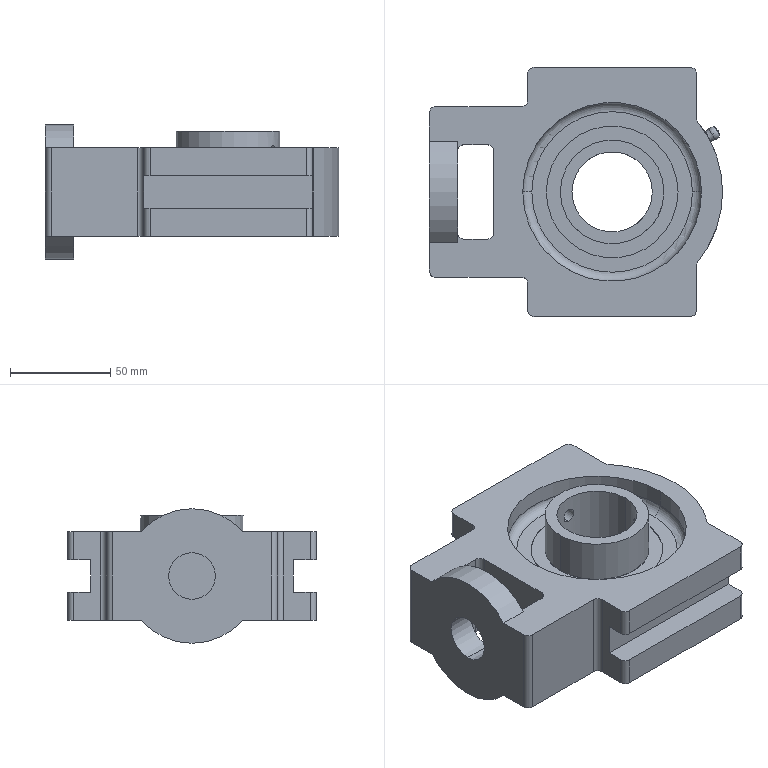Part | STEP file | 1 solid | 124 faces | box 146 x 124 x 67 mm | volume 474066 mm3 | cylinder 48 | plane 34 | sphere 32 | torus 10 | commonest cylinder face diameters 6.222 x18 51.6 x6 65.6 x6 89 x4 67 x3 6.918 x2